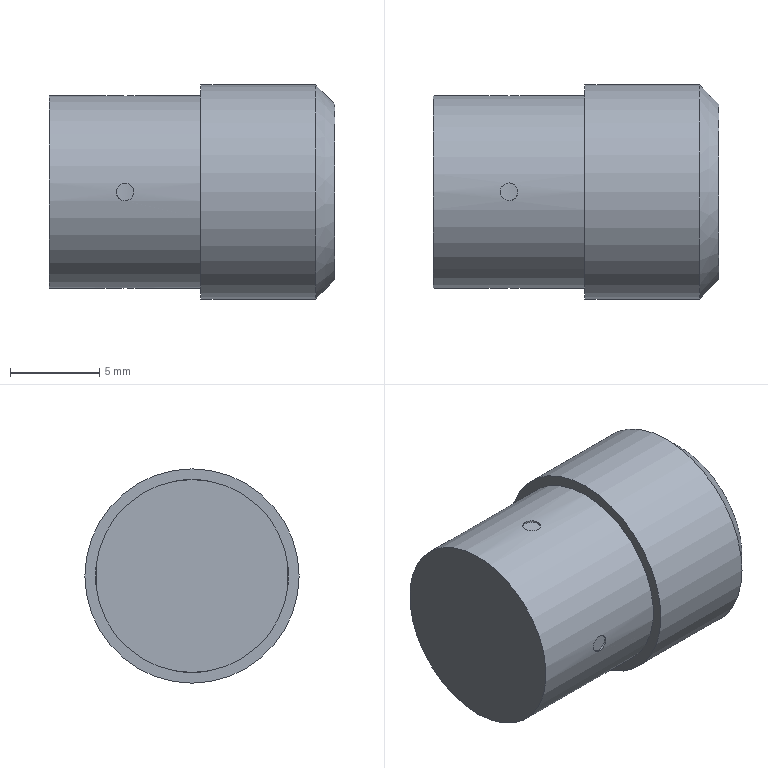Part | NX | features BREP 1 | 1 solid | 24 faces | box 16 x 12 x 12 mm | volume 1191 mm3 | cylinder 15 | plane 8 | cone 1 | commonest cylinder face diameters 1 x8 10.6 x4 9.6 x1 10.8 x1 12 x1
STEP:
#1=CARTESIAN_POINT('',(8.5,0.,5.4));
#2=VERTEX_POINT('',#1);
#3=CARTESIAN_POINT('',(8.5,0.,0.));
#4=DIRECTION('',(-1.,0.,0.));
#5=DIRECTION('',(0.,0.,1.));
#6=AXIS2_PLACEMENT_3D('',#3,#4,#5);
#7=CIRCLE('',#6,5.4);
#8=EDGE_CURVE('',#2,#2,#7,.T.);
#9=ORIENTED_EDGE('',*,*,#8,.T.);
#10=EDGE_LOOP('',(#9));
#11=FACE_BOUND('',#10,.T.);
#12=CARTESIAN_POINT('',(4.75,0.,-5.4));
#13=VERTEX_POINT('',#12);
#14=CARTESIAN_POINT('',(4.249,-0.7501,-5.354));
#15=CARTESIAN_POINT('',(5.,0.00004561,-5.423));
#16=CARTESIAN_POINT('',(4.25,0.7499,-5.354));
#17=CARTESIAN_POINT('',(3.5,0.0003197,-5.423));
#18=CARTESIAN_POINT('',(4.249,-0.7501,-5.354));
#19=CARTESIAN_POINT('',(5.,0.00004561,-5.423));
#20=CARTESIAN_POINT('',(4.25,0.7499,-5.354));
#21=B_SPLINE_CURVE_WITH_KNOTS('',3,(#14,#15,#16,#17,#18,#19,#20),.UNSPECIFIED.,.T.,.F.,(1,1,1,1,1,1,1,1,1,1,1),(-0.002346,-0.001564,-0.0007819,0.,0.0007819,0.001564,0.002346,0.003128,0.00391,0.004692,0.005474),.UNSPECIFIED.);
#22=EDGE_CURVE('',#13,#13,#21,.T.);
#23=ORIENTED_EDGE('',*,*,#22,.T.);
#24=EDGE_LOOP('',(#23));
#25=FACE_BOUND('',#24,.T.);
#26=CARTESIAN_POINT('',(0.,0.,5.4));
#27=VERTEX_POINT('',#26);
#28=CARTESIAN_POINT('',(0.,0.,0.));
#29=DIRECTION('',(1.,0.,0.));
#30=DIRECTION('',(0.,0.,1.));
#31=AXIS2_PLACEMENT_3D('',#28,#29,#30);
#32=CIRCLE('',#31,5.4);
#33=EDGE_CURVE('',#27,#27,#32,.T.);
#34=ORIENTED_EDGE('',*,*,#33,.T.);
#35=EDGE_LOOP('',(#34));
#36=FACE_BOUND('',#35,.T.);
#37=CARTESIAN_POINT('',(4.25,5.377,0.5));
#38=VERTEX_POINT('',#37);
#39=CARTESIAN_POINT('',(5.,5.423,-0.0007741));
#40=CARTESIAN_POINT('',(4.25,5.354,0.7501));
#41=CARTESIAN_POINT('',(3.5,5.423,0.0003559));
#42=CARTESIAN_POINT('',(4.25,5.354,-0.7499));
#43=CARTESIAN_POINT('',(5.,5.423,-0.0007741));
#44=CARTESIAN_POINT('',(4.25,5.354,0.7501));
#45=CARTESIAN_POINT('',(3.5,5.423,0.0003559));
#46=B_SPLINE_CURVE_WITH_KNOTS('',3,(#39,#40,#41,#42,#43,#44,#45),.UNSPECIFIED.,.T.,.F.,(1,1,1,1,1,1,1,1,1,1,1),(-0.002346,-0.001564,-0.0007819,0.,0.0007819,0.001564,0.002346,0.003128,0.00391,0.004692,0.005474),.UNSPECIFIED.);
#47=EDGE_CURVE('',#38,#38,#46,.T.);
#48=ORIENTED_EDGE('',*,*,#47,.T.);
#49=EDGE_LOOP('',(#48));
#50=FACE_BOUND('',#49,.T.);
#51=CARTESIAN_POINT('',(3.75,0.,5.4));
#52=VERTEX_POINT('',#51);
#53=CARTESIAN_POINT('',(4.251,-0.7501,5.354));
#54=CARTESIAN_POINT('',(3.5,0.00004561,5.423));
#55=CARTESIAN_POINT('',(4.25,0.7499,5.354));
#56=CARTESIAN_POINT('',(5.,0.0003197,5.423));
#57=CARTESIAN_POINT('',(4.251,-0.7501,5.354));
#58=CARTESIAN_POINT('',(3.5,0.00004561,5.423));
#59=CARTESIAN_POINT('',(4.25,0.7499,5.354));
#60=B_SPLINE_CURVE_WITH_KNOTS('',3,(#53,#54,#55,#56,#57,#58,#59),.UNSPECIFIED.,.T.,.F.,(1,1,1,1,1,1,1,1,1,1,1),(-0.002346,-0.001564,-0.0007819,0.,0.0007819,0.001564,0.002346,0.003128,0.00391,0.004692,0.005474),.UNSPECIFIED.);
#61=EDGE_CURVE('',#52,#52,#60,.T.);
#62=ORIENTED_EDGE('',*,*,#61,.T.);
#63=EDGE_LOOP('',(#62));
#64=FACE_BOUND('',#63,.T.);
#65=CARTESIAN_POINT('',(4.25,-5.377,-0.5));
#66=VERTEX_POINT('',#65);
#67=CARTESIAN_POINT('',(5.,-5.423,0.0007741));
#68=CARTESIAN_POINT('',(4.25,-5.354,-0.7501));
#69=CARTESIAN_POINT('',(3.5,-5.423,-0.0003559));
#70=CARTESIAN_POINT('',(4.25,-5.354,0.7499));
#71=CARTESIAN_POINT('',(5.,-5.423,0.0007741));
#72=CARTESIAN_POINT('',(4.25,-5.354,-0.7501));
#73=CARTESIAN_POINT('',(3.5,-5.423,-0.0003559));
#74=B_SPLINE_CURVE_WITH_KNOTS('',3,(#67,#68,#69,#70,#71,#72,#73),.UNSPECIFIED.,.T.,.F.,(1,1,1,1,1,1,1,1,1,1,1),(-0.002346,-0.001564,-0.0007819,0.,0.0007819,0.001564,0.002346,0.003128,0.00391,0.004692,0.005474),.UNSPECIFIED.);
#75=EDGE_CURVE('',#66,#66,#74,.T.);
#76=ORIENTED_EDGE('',*,*,#75,.T.);
#77=EDGE_LOOP('',(#76));
#78=FACE_BOUND('',#77,.T.);
#79=CARTESIAN_POINT('',(8.5,0.,0.));
#80=DIRECTION('',(-1.,0.,0.));
#81=DIRECTION('',(0.,0.,-1.));
#82=AXIS2_PLACEMENT_3D('',#79,#80,#81);
#83=CYLINDRICAL_SURFACE('',#82,5.4);
#84=ADVANCED_FACE('',(#11,#25,#36,#50,#64,#78),#83,.T.);
#85=ORIENTED_EDGE('',*,*,#47,.F.);
#86=EDGE_LOOP('',(#85));
#87=FACE_BOUND('',#86,.T.);
#88=CARTESIAN_POINT('',(4.25,5.276,0.5));
#89=VERTEX_POINT('',#88);
#90=CARTESIAN_POINT('',(3.5,5.324,-0.0007718));
#91=CARTESIAN_POINT('',(4.25,5.253,0.7501));
#92=CARTESIAN_POINT('',(5.,5.324,0.0003567));
#93=CARTESIAN_POINT('',(4.25,5.253,-0.7499));
#94=CARTESIAN_POINT('',(3.5,5.324,-0.0007718));
#95=CARTESIAN_POINT('',(4.25,5.253,0.7501));
#96=CARTESIAN_POINT('',(5.,5.324,0.0003567));
#97=B_SPLINE_CURVE_WITH_KNOTS('',3,(#90,#91,#92,#93,#94,#95,#96),.UNSPECIFIED.,.T.,.F.,(1,1,1,1,1,1,1,1,1,1,1),(-0.002346,-0.001564,-0.000782,0.,0.000782,0.001564,0.002346,0.003128,0.00391,0.004692,0.005474),.UNSPECIFIED.);
#98=EDGE_CURVE('',#89,#89,#97,.T.);
#99=ORIENTED_EDGE('',*,*,#98,.F.);
#100=EDGE_LOOP('',(#99));
#101=FACE_BOUND('',#100,.T.);
#102=CARTESIAN_POINT('',(4.25,0.,0.));
#103=DIRECTION('',(0.,1.,0.));
#104=DIRECTION('',(0.,0.,-1.));
#105=AXIS2_PLACEMENT_3D('',#102,#103,#104);
#106=CYLINDRICAL_SURFACE('',#105,0.5);
#107=ADVANCED_FACE('',(#87,#101),#106,.F.);
#108=CARTESIAN_POINT('',(4.75,0.,5.3));
#109=VERTEX_POINT('',#108);
#110=CARTESIAN_POINT('',(4.249,-0.7501,5.253));
#111=CARTESIAN_POINT('',(5.,0.00004567,5.324));
#112=CARTESIAN_POINT('',(4.25,0.7499,5.253));
#113=CARTESIAN_POINT('',(3.5,0.0003201,5.324));
#114=CARTESIAN_POINT('',(4.249,-0.7501,5.253));
#115=CARTESIAN_POINT('',(5.,0.00004567,5.324));
#116=CARTESIAN_POINT('',(4.25,0.7499,5.253));
#117=B_SPLINE_CURVE_WITH_KNOTS('',3,(#110,#111,#112,#113,#114,#115,#116),.UNSPECIFIED.,.T.,.F.,(1,1,1,1,1,1,1,1,1,1,1),(-0.002346,-0.001564,-0.000782,0.,0.000782,0.001564,0.002346,0.003128,0.00391,0.004692,0.005474),.UNSPECIFIED.);
#118=EDGE_CURVE('',#109,#109,#117,.T.);
#119=ORIENTED_EDGE('',*,*,#118,.F.);
#120=EDGE_LOOP('',(#119));
#121=FACE_BOUND('',#120,.T.);
#122=ORIENTED_EDGE('',*,*,#61,.F.);
#123=EDGE_LOOP('',(#122));
#124=FACE_BOUND('',#123,.T.);
#125=CARTESIAN_POINT('',(4.25,0.,5.4));
#126=DIRECTION('',(0.,0.,-1.));
#127=DIRECTION('',(1.,0.,0.));
#128=AXIS2_PLACEMENT_3D('',#125,#126,#127);
#129=CYLINDRICAL_SURFACE('',#128,0.5);
#130=ADVANCED_FACE('',(#121,#124),#129,.F.);
#131=ORIENTED_EDGE('',*,*,#33,.F.);
#132=EDGE_LOOP('',(#131));
#133=FACE_BOUND('',#132,.T.);
#134=CARTESIAN_POINT('',(0.,0.,0.));
#135=DIRECTION('',(1.,0.,0.));
#136=DIRECTION('',(0.,0.,1.));
#137=AXIS2_PLACEMENT_3D('',#134,#135,#136);
#138=PLANE('',#137);
#139=ADVANCED_FACE('',(#133),#138,.F.);
#140=ORIENTED_EDGE('',*,*,#22,.F.);
#141=EDGE_LOOP('',(#140));
#142=FACE_BOUND('',#141,.T.);
#143=CARTESIAN_POINT('',(3.75,0.,-5.3));
#144=VERTEX_POINT('',#143);
#145=CARTESIAN_POINT('',(4.251,-0.7501,-5.253));
#146=CARTESIAN_POINT('',(3.5,0.00004567,-5.324));
#147=CARTESIAN_POINT('',(4.25,0.7499,-5.253));
#148=CARTESIAN_POINT('',(5.,0.0003201,-5.324));
#149=CARTESIAN_POINT('',(4.251,-0.7501,-5.253));
#150=CARTESIAN_POINT('',(3.5,0.00004567,-5.324));
#151=CARTESIAN_POINT('',(4.25,0.7499,-5.253));
#152=B_SPLINE_CURVE_WITH_KNOTS('',3,(#145,#146,#147,#148,#149,#150,#151),.UNSPECIFIED.,.T.,.F.,(1,1,1,1,1,1,1,1,1,1,1),(-0.002346,-0.001564,-0.000782,0.,0.000782,0.001564,0.002346,0.003128,0.00391,0.004692,0.005474),.UNSPECIFIED.);
#153=EDGE_CURVE('',#144,#144,#152,.T.);
#154=ORIENTED_EDGE('',*,*,#153,.F.);
#155=EDGE_LOOP('',(#154));
#156=FACE_BOUND('',#155,.T.);
#157=CARTESIAN_POINT('',(4.25,0.,0.));
#158=DIRECTION('',(0.,0.,-1.));
#159=DIRECTION('',(1.,0.,0.));
#160=AXIS2_PLACEMENT_3D('',#157,#158,#159);
#161=CYLINDRICAL_SURFACE('',#160,0.5);
#162=ADVANCED_FACE('',(#142,#156),#161,.F.);
#163=CARTESIAN_POINT('',(8.5,0.,6.));
#164=VERTEX_POINT('',#163);
#165=CARTESIAN_POINT('',(8.5,0.,0.));
#166=DIRECTION('',(1.,0.,0.));
#167=DIRECTION('',(0.,0.,1.));
#168=AXIS2_PLACEMENT_3D('',#165,#166,#167);
#169=CIRCLE('',#168,6.);
#170=EDGE_CURVE('',#164,#164,#169,.T.);
#171=ORIENTED_EDGE('',*,*,#170,.F.);
#172=EDGE_LOOP('',(#171));
#173=FACE_BOUND('',#172,.T.);
#174=ORIENTED_EDGE('',*,*,#8,.F.);
#175=EDGE_LOOP('',(#174));
#176=FACE_BOUND('',#175,.T.);
#177=CARTESIAN_POINT('',(8.5,0.,0.));
#178=DIRECTION('',(1.,0.,0.));
#179=DIRECTION('',(0.,0.,1.));
#180=AXIS2_PLACEMENT_3D('',#177,#178,#179);
#181=PLANE('',#180);
#182=ADVANCED_FACE('',(#173,#176),#181,.F.);
#183=ORIENTED_EDGE('',*,*,#98,.T.);
#184=EDGE_LOOP('',(#183));
#185=FACE_BOUND('',#184,.T.);
#186=CARTESIAN_POINT('',(8.5,0.,0.));
#187=DIRECTION('',(-1.,0.,0.));
#188=DIRECTION('',(0.,0.,-1.));
#189=AXIS2_PLACEMENT_3D('',#186,#187,#188);
#190=CYLINDRICAL_SURFACE('',#189,5.3);
#191=ADVANCED_FACE('',(#185),#190,.T.);
#192=ORIENTED_EDGE('',*,*,#118,.T.);
#193=EDGE_LOOP('',(#192));
#194=FACE_BOUND('',#193,.T.);
#195=CARTESIAN_POINT('',(8.5,0.,0.));
#196=DIRECTION('',(-1.,0.,0.));
#197=DIRECTION('',(0.,0.,-1.));
#198=AXIS2_PLACEMENT_3D('',#195,#196,#197);
#199=CYLINDRICAL_SURFACE('',#198,5.3);
#200=ADVANCED_FACE('',(#194),#199,.T.);
#201=ORIENTED_EDGE('',*,*,#75,.F.);
#202=EDGE_LOOP('',(#201));
#203=FACE_BOUND('',#202,.T.);
#204=CARTESIAN_POINT('',(4.25,-5.276,0.5));
#205=VERTEX_POINT('',#204);
#206=CARTESIAN_POINT('',(5.,-5.324,-0.0007718));
#207=CARTESIAN_POINT('',(4.25,-5.253,0.7501));
#208=CARTESIAN_POINT('',(3.5,-5.324,0.0003567));
#209=CARTESIAN_POINT('',(4.25,-5.253,-0.7499));
#210=CARTESIAN_POINT('',(5.,-5.324,-0.0007718));
#211=CARTESIAN_POINT('',(4.25,-5.253,0.7501));
#212=CARTESIAN_POINT('',(3.5,-5.324,0.0003567));
#213=B_SPLINE_CURVE_WITH_KNOTS('',3,(#206,#207,#208,#209,#210,#211,#212),.UNSPECIFIED.,.T.,.F.,(1,1,1,1,1,1,1,1,1,1,1),(-0.002346,-0.001564,-0.000782,0.,0.000782,0.001564,0.002346,0.003128,0.00391,0.004692,0.005474),.UNSPECIFIED.);
#214=EDGE_CURVE('',#205,#205,#213,.T.);
#215=ORIENTED_EDGE('',*,*,#214,.F.);
#216=EDGE_LOOP('',(#215));
#217=FACE_BOUND('',#216,.T.);
#218=CARTESIAN_POINT('',(4.25,0.,0.));
#219=DIRECTION('',(0.,1.,0.));
#220=DIRECTION('',(0.,0.,-1.));
#221=AXIS2_PLACEMENT_3D('',#218,#219,#220);
#222=CYLINDRICAL_SURFACE('',#221,0.5);
#223=ADVANCED_FACE('',(#203,#217),#222,.F.);
#224=ORIENTED_EDGE('',*,*,#153,.T.);
#225=EDGE_LOOP('',(#224));
#226=FACE_BOUND('',#225,.T.);
#227=CARTESIAN_POINT('',(8.5,0.,0.));
#228=DIRECTION('',(-1.,0.,0.));
#229=DIRECTION('',(0.,0.,-1.));
#230=AXIS2_PLACEMENT_3D('',#227,#228,#229);
#231=CYLINDRICAL_SURFACE('',#230,5.3);
#232=ADVANCED_FACE('',(#226),#231,.T.);
#233=CARTESIAN_POINT('',(14.927,0.,6.));
#234=VERTEX_POINT('',#233);
#235=CARTESIAN_POINT('',(14.927,0.,0.));
#236=DIRECTION('',(-1.,0.,0.));
#237=DIRECTION('',(0.,0.,1.));
#238=AXIS2_PLACEMENT_3D('',#235,#236,#237);
#239=CIRCLE('',#238,6.);
#240=EDGE_CURVE('',#234,#234,#239,.T.);
#241=ORIENTED_EDGE('',*,*,#240,.T.);
#242=EDGE_LOOP('',(#241));
#243=FACE_BOUND('',#242,.T.);
#244=ORIENTED_EDGE('',*,*,#170,.T.);
#245=EDGE_LOOP('',(#244));
#246=FACE_BOUND('',#245,.T.);
#247=CARTESIAN_POINT('',(16.,0.,0.));
#248=DIRECTION('',(-1.,0.,0.));
#249=DIRECTION('',(0.,0.,-1.));
#250=AXIS2_PLACEMENT_3D('',#247,#248,#249);
#251=CYLINDRICAL_SURFACE('',#250,6.);
#252=ADVANCED_FACE('',(#243,#246),#251,.T.);
#253=ORIENTED_EDGE('',*,*,#214,.T.);
#254=EDGE_LOOP('',(#253));
#255=FACE_BOUND('',#254,.T.);
#256=CARTESIAN_POINT('',(8.5,0.,0.));
#257=DIRECTION('',(-1.,0.,0.));
#258=DIRECTION('',(0.,0.,-1.));
#259=AXIS2_PLACEMENT_3D('',#256,#257,#258);
#260=CYLINDRICAL_SURFACE('',#259,5.3);
#261=ADVANCED_FACE('',(#255),#260,.T.);
#262=ORIENTED_EDGE('',*,*,#240,.F.);
#263=EDGE_LOOP('',(#262));
#264=FACE_BOUND('',#263,.T.);
#265=CARTESIAN_POINT('',(16.,0.,4.927));
#266=VERTEX_POINT('',#265);
#267=CARTESIAN_POINT('',(16.,0.,0.));
#268=DIRECTION('',(-1.,0.,0.));
#269=DIRECTION('',(0.,0.,1.));
#270=AXIS2_PLACEMENT_3D('',#267,#268,#269);
#271=CIRCLE('',#270,4.927);
#272=EDGE_CURVE('',#266,#266,#271,.T.);
#273=ORIENTED_EDGE('',*,*,#272,.T.);
#274=EDGE_LOOP('',(#273));
#275=FACE_BOUND('',#274,.T.);
#276=CARTESIAN_POINT('',(14.927,0.,0.));
#277=DIRECTION('',(-1.,0.,0.));
#278=DIRECTION('',(0.,0.,-1.));
#279=AXIS2_PLACEMENT_3D('',#276,#277,#278);
#280=CONICAL_SURFACE('',#279,6.,0.7854);
#281=ADVANCED_FACE('',(#264,#275),#280,.T.);
#282=ORIENTED_EDGE('',*,*,#272,.F.);
#283=EDGE_LOOP('',(#282));
#284=FACE_BOUND('',#283,.T.);
#285=CARTESIAN_POINT('',(16.,0.,4.8));
#286=VERTEX_POINT('',#285);
#287=CARTESIAN_POINT('',(16.,0.,0.));
#288=DIRECTION('',(1.,0.,0.));
#289=DIRECTION('',(0.,0.,1.));
#290=AXIS2_PLACEMENT_3D('',#287,#288,#289);
#291=CIRCLE('',#290,4.8);
#292=EDGE_CURVE('',#286,#286,#291,.T.);
#293=ORIENTED_EDGE('',*,*,#292,.F.);
#294=EDGE_LOOP('',(#293));
#295=FACE_BOUND('',#294,.T.);
#296=CARTESIAN_POINT('',(16.,4.926,0.));
#297=DIRECTION('',(-1.,0.,0.));
#298=DIRECTION('',(0.,0.,-1.));
#299=AXIS2_PLACEMENT_3D('',#296,#297,#298);
#300=PLANE('',#299);
#301=ADVANCED_FACE('',(#284,#295),#300,.F.);
#302=CARTESIAN_POINT('',(10.,0.,4.8));
#303=VERTEX_POINT('',#302);
#304=CARTESIAN_POINT('',(10.,0.,0.));
#305=DIRECTION('',(1.,0.,0.));
#306=DIRECTION('',(0.,0.,1.));
#307=AXIS2_PLACEMENT_3D('',#304,#305,#306);
#308=CIRCLE('',#307,4.8);
#309=EDGE_CURVE('',#303,#303,#308,.T.);
#310=ORIENTED_EDGE('',*,*,#309,.F.);
#311=EDGE_LOOP('',(#310));
#312=FACE_BOUND('',#311,.T.);
#313=ORIENTED_EDGE('',*,*,#292,.T.);
#314=EDGE_LOOP('',(#313));
#315=FACE_BOUND('',#314,.T.);
#316=CARTESIAN_POINT('',(10.,0.,0.));
#317=DIRECTION('',(-1.,0.,0.));
#318=DIRECTION('',(0.,0.,-1.));
#319=AXIS2_PLACEMENT_3D('',#316,#317,#318);
#320=CYLINDRICAL_SURFACE('',#319,4.8);
#321=ADVANCED_FACE('',(#312,#315),#320,.F.);
#322=ORIENTED_EDGE('',*,*,#309,.T.);
#323=EDGE_LOOP('',(#322));
#324=FACE_BOUND('',#323,.T.);
#325=CARTESIAN_POINT('',(10.,0.,2.9));
#326=VERTEX_POINT('',#325);
#327=CARTESIAN_POINT('',(10.,0.,2.4));
#328=DIRECTION('',(-1.,0.,0.));
#329=DIRECTION('',(0.,0.,1.));
#330=AXIS2_PLACEMENT_3D('',#327,#328,#329);
#331=CIRCLE('',#330,0.5);
#332=EDGE_CURVE('',#326,#326,#331,.T.);
#333=ORIENTED_EDGE('',*,*,#332,.T.);
#334=EDGE_LOOP('',(#333));
#335=FACE_BOUND('',#334,.T.);
#336=CARTESIAN_POINT('',(10.,-2.4,0.5));
#337=VERTEX_POINT('',#336);
#338=CARTESIAN_POINT('',(10.,-2.4,0.));
#339=DIRECTION('',(-1.,0.,0.));
#340=DIRECTION('',(0.,0.,1.));
#341=AXIS2_PLACEMENT_3D('',#338,#339,#340);
#342=CIRCLE('',#341,0.5);
#343=EDGE_CURVE('',#337,#337,#342,.T.);
#344=ORIENTED_EDGE('',*,*,#343,.T.);
#345=EDGE_LOOP('',(#344));
#346=FACE_BOUND('',#345,.T.);
#347=CARTESIAN_POINT('',(10.,2.4,0.5));
#348=VERTEX_POINT('',#347);
#349=CARTESIAN_POINT('',(10.,2.4,0.));
#350=DIRECTION('',(-1.,0.,0.));
#351=DIRECTION('',(0.,0.,1.));
#352=AXIS2_PLACEMENT_3D('',#349,#350,#351);
#353=CIRCLE('',#352,0.5);
#354=EDGE_CURVE('',#348,#348,#353,.T.);
#355=ORIENTED_EDGE('',*,*,#354,.T.);
#356=EDGE_LOOP('',(#355));
#357=FACE_BOUND('',#356,.T.);
#358=CARTESIAN_POINT('',(10.,0.,-1.9));
#359=VERTEX_POINT('',#358);
#360=CARTESIAN_POINT('',(10.,0.,-2.4));
#361=DIRECTION('',(-1.,0.,0.));
#362=DIRECTION('',(0.,0.,1.));
#363=AXIS2_PLACEMENT_3D('',#360,#361,#362);
#364=CIRCLE('',#363,0.5);
#365=EDGE_CURVE('',#359,#359,#364,.T.);
#366=ORIENTED_EDGE('',*,*,#365,.T.);
#367=EDGE_LOOP('',(#366));
#368=FACE_BOUND('',#367,.T.);
#369=CARTESIAN_POINT('',(10.,0.,0.));
#370=DIRECTION('',(1.,0.,0.));
#371=DIRECTION('',(0.,0.,1.));
#372=AXIS2_PLACEMENT_3D('',#369,#370,#371);
#373=PLANE('',#372);
#374=ADVANCED_FACE('',(#324,#335,#346,#357,#368),#373,.T.);
#375=ORIENTED_EDGE('',*,*,#332,.F.);
#376=EDGE_LOOP('',(#375));
#377=FACE_BOUND('',#376,.T.);
#378=CARTESIAN_POINT('',(16.,0.,2.9));
#379=VERTEX_POINT('',#378);
#380=CARTESIAN_POINT('',(16.,0.,2.4));
#381=DIRECTION('',(-1.,0.,0.));
#382=DIRECTION('',(0.,0.,1.));
#383=AXIS2_PLACEMENT_3D('',#380,#381,#382);
#384=CIRCLE('',#383,0.5);
#385=EDGE_CURVE('',#379,#379,#384,.T.);
#386=ORIENTED_EDGE('',*,*,#385,.T.);
#387=EDGE_LOOP('',(#386));
#388=FACE_BOUND('',#387,.T.);
#389=CARTESIAN_POINT('',(10.,0.,2.4));
#390=DIRECTION('',(-1.,0.,0.));
#391=DIRECTION('',(0.,0.,-1.));
#392=AXIS2_PLACEMENT_3D('',#389,#390,#391);
#393=CYLINDRICAL_SURFACE('',#392,0.5);
#394=ADVANCED_FACE('',(#377,#388),#393,.T.);
#395=ORIENTED_EDGE('',*,*,#343,.F.);
#396=EDGE_LOOP('',(#395));
#397=FACE_BOUND('',#396,.T.);
#398=CARTESIAN_POINT('',(16.,-2.4,0.5));
#399=VERTEX_POINT('',#398);
#400=CARTESIAN_POINT('',(16.,-2.4,0.));
#401=DIRECTION('',(-1.,0.,0.));
#402=DIRECTION('',(0.,0.,1.));
#403=AXIS2_PLACEMENT_3D('',#400,#401,#402);
#404=CIRCLE('',#403,0.5);
#405=EDGE_CURVE('',#399,#399,#404,.T.);
#406=ORIENTED_EDGE('',*,*,#405,.T.);
#407=EDGE_LOOP('',(#406));
#408=FACE_BOUND('',#407,.T.);
#409=CARTESIAN_POINT('',(10.,-2.4,0.));
#410=DIRECTION('',(-1.,0.,0.));
#411=DIRECTION('',(0.,0.,-1.));
#412=AXIS2_PLACEMENT_3D('',#409,#410,#411);
#413=CYLINDRICAL_SURFACE('',#412,0.5);
#414=ADVANCED_FACE('',(#397,#408),#413,.T.);
#415=ORIENTED_EDGE('',*,*,#354,.F.);
#416=EDGE_LOOP('',(#415));
#417=FACE_BOUND('',#416,.T.);
#418=CARTESIAN_POINT('',(16.,2.4,0.5));
#419=VERTEX_POINT('',#418);
#420=CARTESIAN_POINT('',(16.,2.4,0.));
#421=DIRECTION('',(-1.,0.,0.));
#422=DIRECTION('',(0.,0.,1.));
#423=AXIS2_PLACEMENT_3D('',#420,#421,#422);
#424=CIRCLE('',#423,0.5);
#425=EDGE_CURVE('',#419,#419,#424,.T.);
#426=ORIENTED_EDGE('',*,*,#425,.T.);
#427=EDGE_LOOP('',(#426));
#428=FACE_BOUND('',#427,.T.);
#429=CARTESIAN_POINT('',(10.,2.4,0.));
#430=DIRECTION('',(-1.,0.,0.));
#431=DIRECTION('',(0.,0.,-1.));
#432=AXIS2_PLACEMENT_3D('',#429,#430,#431);
#433=CYLINDRICAL_SURFACE('',#432,0.5);
#434=ADVANCED_FACE('',(#417,#428),#433,.T.);
#435=ORIENTED_EDGE('',*,*,#365,.F.);
#436=EDGE_LOOP('',(#435));
#437=FACE_BOUND('',#436,.T.);
#438=CARTESIAN_POINT('',(16.,0.,-1.9));
#439=VERTEX_POINT('',#438);
#440=CARTESIAN_POINT('',(16.,0.,-2.4));
#441=DIRECTION('',(-1.,0.,0.));
#442=DIRECTION('',(0.,0.,1.));
#443=AXIS2_PLACEMENT_3D('',#440,#441,#442);
#444=CIRCLE('',#443,0.5);
#445=EDGE_CURVE('',#439,#439,#444,.T.);
#446=ORIENTED_EDGE('',*,*,#445,.T.);
#447=EDGE_LOOP('',(#446));
#448=FACE_BOUND('',#447,.T.);
#449=CARTESIAN_POINT('',(10.,0.,-2.4));
#450=DIRECTION('',(-1.,0.,0.));
#451=DIRECTION('',(0.,0.,-1.));
#452=AXIS2_PLACEMENT_3D('',#449,#450,#451);
#453=CYLINDRICAL_SURFACE('',#452,0.5);
#454=ADVANCED_FACE('',(#437,#448),#453,.T.);
#455=ORIENTED_EDGE('',*,*,#385,.F.);
#456=EDGE_LOOP('',(#455));
#457=FACE_BOUND('',#456,.T.);
#458=CARTESIAN_POINT('',(16.,4.926,0.));
#459=DIRECTION('',(-1.,0.,0.));
#460=DIRECTION('',(0.,0.,-1.));
#461=AXIS2_PLACEMENT_3D('',#458,#459,#460);
#462=PLANE('',#461);
#463=ADVANCED_FACE('',(#457),#462,.F.);
#464=ORIENTED_EDGE('',*,*,#405,.F.);
#465=EDGE_LOOP('',(#464));
#466=FACE_BOUND('',#465,.T.);
#467=CARTESIAN_POINT('',(16.,4.926,0.));
#468=DIRECTION('',(-1.,0.,0.));
#469=DIRECTION('',(0.,0.,-1.));
#470=AXIS2_PLACEMENT_3D('',#467,#468,#469);
#471=PLANE('',#470);
#472=ADVANCED_FACE('',(#466),#471,.F.);
#473=ORIENTED_EDGE('',*,*,#425,.F.);
#474=EDGE_LOOP('',(#473));
#475=FACE_BOUND('',#474,.T.);
#476=CARTESIAN_POINT('',(16.,4.926,0.));
#477=DIRECTION('',(-1.,0.,0.));
#478=DIRECTION('',(0.,0.,-1.));
#479=AXIS2_PLACEMENT_3D('',#476,#477,#478);
#480=PLANE('',#479);
#481=ADVANCED_FACE('',(#475),#480,.F.);
#482=ORIENTED_EDGE('',*,*,#445,.F.);
#483=EDGE_LOOP('',(#482));
#484=FACE_BOUND('',#483,.T.);
#485=CARTESIAN_POINT('',(16.,4.926,0.));
#486=DIRECTION('',(-1.,0.,0.));
#487=DIRECTION('',(0.,0.,-1.));
#488=AXIS2_PLACEMENT_3D('',#485,#486,#487);
#489=PLANE('',#488);
#490=ADVANCED_FACE('',(#484),#489,.F.);
#491=CLOSED_SHELL('',(#84,#107,#130,#139,#162,#182,#191,#200,#223,#232,#252,#261,#281,#301,#321,#374,#394,#414,#434,#454,#463,#472,#481,#490));
#492=MANIFOLD_SOLID_BREP('',#491);
#493=(LENGTH_UNIT()NAMED_UNIT(*)SI_UNIT(.MILLI.,.METRE.));
#494=UNCERTAINTY_MEASURE_WITH_UNIT(LENGTH_MEASURE(0.0508),#493,'','');
#495=(NAMED_UNIT(*)PLANE_ANGLE_UNIT()SI_UNIT($,.RADIAN.));
#496=(NAMED_UNIT(*)SI_UNIT($,.STERADIAN.)SOLID_ANGLE_UNIT());
#497=(GEOMETRIC_REPRESENTATION_CONTEXT(3)GLOBAL_UNCERTAINTY_ASSIGNED_CONTEXT((#494))GLOBAL_UNIT_ASSIGNED_CONTEXT((#493,#495,#496))REPRESENTATION_CONTEXT('',''));
#498=ADVANCED_BREP_SHAPE_REPRESENTATION('',(#492),#497);